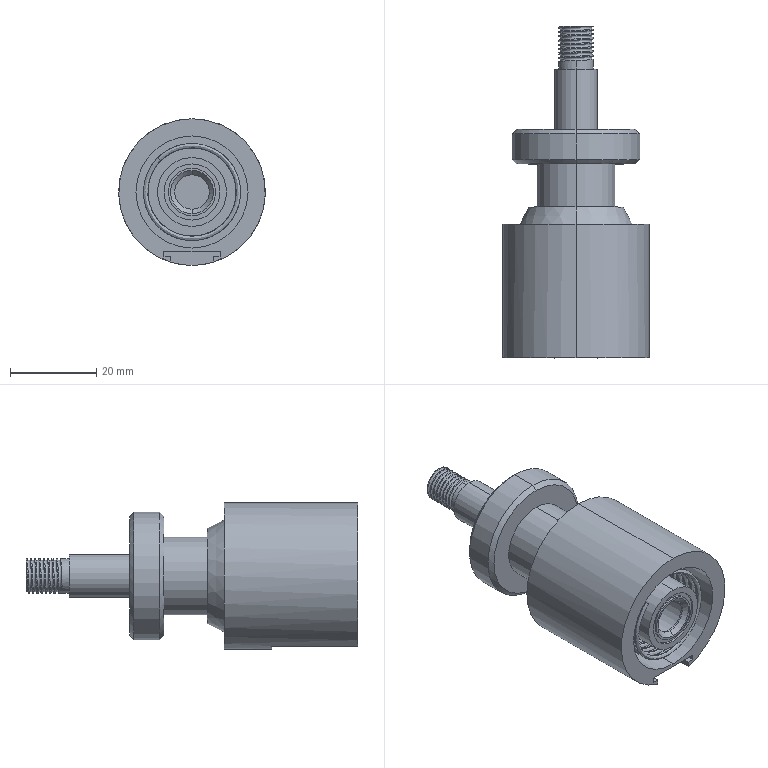Part | SolidWorks | features ICE 29, RevCut 6, Chamfer 4, Helix 2, Extrusion 1, Sweep 1, SweepCut 1 | 1 solid | 84 faces | box 34 x 77 x 34 mm | volume 30260 mm3 | cylinder 43 | plane 26 | cone 12 | spline 3 | commonest cylinder face diameters 8 x19 11 x4 9.608 x2 10 x2 12.482 x2 13 x2